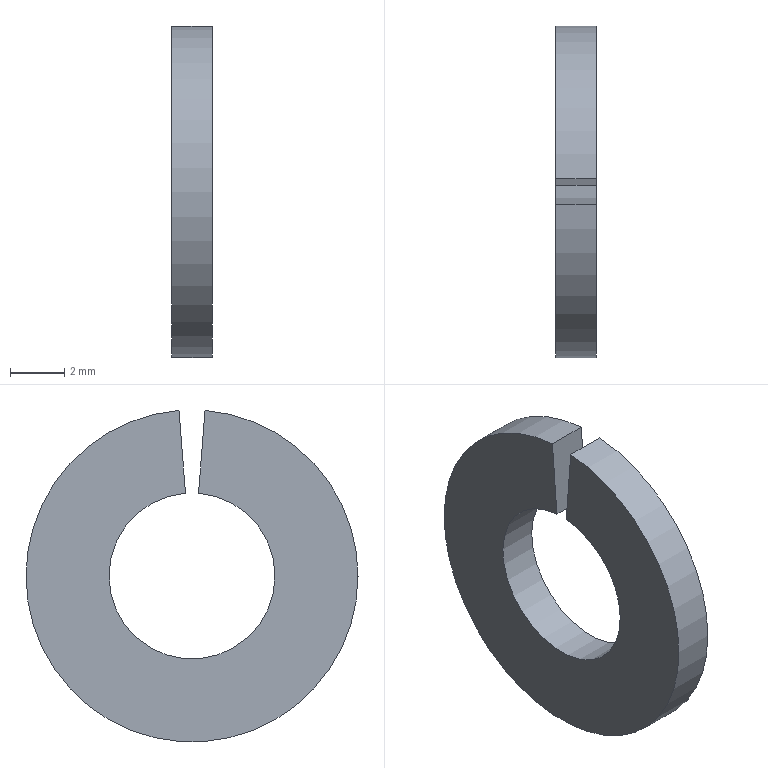Part | STEP file | PN_0038_default | 1 solid | 6 faces | box 1.5 x 12.2 x 12.181 mm | volume 128.223 mm3 | plane 4 | cylinder 2 | commonest cylinder face diameters 6.1 x1 12.2 x1
STEP:
#1=CARTESIAN_POINT('',(0.,0.,0.));
#2=DIRECTION('',(0.,0.,1.));
#3=DIRECTION('',(1.,0.,0.));
#4=AXIS2_PLACEMENT_3D('',#1,#2,#3);
#5=CARTESIAN_POINT('',(0.,0.2393,3.041));
#6=VERTEX_POINT('',#5);
#7=CARTESIAN_POINT('',(0.,0.4786,6.081));
#8=VERTEX_POINT('',#7);
#9=CARTESIAN_POINT('',(0.,0.2393,3.041));
#10=DIRECTION('',(0.,0.07846,0.9969));
#11=VECTOR('',#10,1.);
#12=LINE('',#9,#11);
#13=CARTESIAN_POINT('',(0.,3.05,0.));
#14=DIRECTION('',(-1.,0.,0.));
#15=DIRECTION('',(0.,0.,1.));
#16=AXIS2_PLACEMENT_3D('',#13,#14,#15);
#17=PLANE('',#16);
#18=CARTESIAN_POINT('',(3.041,-2.811));
#19=DIRECTION('',(0.9969,0.07846));
#20=VECTOR('',#19,1.);
#21=LINE('',#18,#20);
#22=(GEOMETRIC_REPRESENTATION_CONTEXT(2)PARAMETRIC_REPRESENTATION_CONTEXT()REPRESENTATION_CONTEXT('',''));
#23=DEFINITIONAL_REPRESENTATION('',(#21),#22);
#24=PCURVE('',#17,#23);
#25=CARTESIAN_POINT('',(-1.5,0.,0.));
#26=DIRECTION('',(0.,0.9969,-0.07846));
#27=DIRECTION('',(0.,0.07846,0.9969));
#28=AXIS2_PLACEMENT_3D('',#25,#26,#27);
#29=PLANE('',#28);
#30=CARTESIAN_POINT('',(3.05,1.5));
#31=DIRECTION('',(1.,0.));
#32=VECTOR('',#31,1.);
#33=LINE('',#30,#32);
#34=(GEOMETRIC_REPRESENTATION_CONTEXT(2)PARAMETRIC_REPRESENTATION_CONTEXT()REPRESENTATION_CONTEXT('',''));
#35=DEFINITIONAL_REPRESENTATION('',(#33),#34);
#36=PCURVE('',#29,#35);
#37=SURFACE_CURVE('',#12,(#24,#36),.PCURVE_S1.);
#38=EDGE_CURVE('',#6,#8,#37,.T.);
#39=ORIENTED_EDGE('',*,*,#38,.F.);
#40=CARTESIAN_POINT('',(0.,-0.2393,3.041));
#41=VERTEX_POINT('',#40);
#42=CARTESIAN_POINT('',(0.,0.,0.));
#43=DIRECTION('',(1.,0.,0.));
#44=DIRECTION('',(0.,0.,1.));
#45=AXIS2_PLACEMENT_3D('',#42,#43,#44);
#46=CIRCLE('',#45,3.05);
#47=CARTESIAN_POINT('',(3.05,-3.05));
#48=CARTESIAN_POINT('',(3.05,-8.333));
#49=CARTESIAN_POINT('',(-1.525,-5.691));
#50=CARTESIAN_POINT('',(-6.1,-3.05));
#51=CARTESIAN_POINT('',(-1.525,-0.4086));
#52=CARTESIAN_POINT('',(3.05,2.233));
#53=CARTESIAN_POINT('',(3.05,-3.05));
#54=(BOUNDED_CURVE()B_SPLINE_CURVE(2,(#47,#48,#49,#50,#51,#52,#53),.UNSPECIFIED.,.T.,.F.)B_SPLINE_CURVE_WITH_KNOTS((1,2,2,2,2,1),(-2.094,0.,2.094,4.189,6.283,8.378),.UNSPECIFIED.)CURVE()GEOMETRIC_REPRESENTATION_ITEM()RATIONAL_B_SPLINE_CURVE((1.,0.5,1.,0.5,1.,0.5,1.))REPRESENTATION_ITEM(''));
#55=(GEOMETRIC_REPRESENTATION_CONTEXT(2)PARAMETRIC_REPRESENTATION_CONTEXT()REPRESENTATION_CONTEXT('',''));
#56=DEFINITIONAL_REPRESENTATION('',(#54),#55);
#57=PCURVE('',#17,#56);
#58=CARTESIAN_POINT('',(-34.925,0.,0.));
#59=DIRECTION('',(-1.,0.,0.));
#60=DIRECTION('',(0.,0.,1.));
#61=AXIS2_PLACEMENT_3D('',#58,#59,#60);
#62=CYLINDRICAL_SURFACE('',#61,3.05);
#63=CARTESIAN_POINT('',(6.283,-34.925));
#64=DIRECTION('',(-1.,0.));
#65=VECTOR('',#64,1.);
#66=LINE('',#63,#65);
#67=(GEOMETRIC_REPRESENTATION_CONTEXT(2)PARAMETRIC_REPRESENTATION_CONTEXT()REPRESENTATION_CONTEXT('',''));
#68=DEFINITIONAL_REPRESENTATION('',(#66),#67);
#69=PCURVE('',#62,#68);
#70=SURFACE_CURVE('',#46,(#57,#69),.PCURVE_S1.);
#71=EDGE_CURVE('',#41,#6,#70,.T.);
#72=ORIENTED_EDGE('',*,*,#71,.F.);
#73=CARTESIAN_POINT('',(0.,-0.4786,6.081));
#74=VERTEX_POINT('',#73);
#75=CARTESIAN_POINT('',(0.,-0.4786,6.081));
#76=DIRECTION('',(0.,0.07846,-0.9969));
#77=VECTOR('',#76,1.);
#78=LINE('',#75,#77);
#79=CARTESIAN_POINT('',(6.081,-3.529));
#80=DIRECTION('',(-0.9969,0.07846));
#81=VECTOR('',#80,1.);
#82=LINE('',#79,#81);
#83=(GEOMETRIC_REPRESENTATION_CONTEXT(2)PARAMETRIC_REPRESENTATION_CONTEXT()REPRESENTATION_CONTEXT('',''));
#84=DEFINITIONAL_REPRESENTATION('',(#82),#83);
#85=PCURVE('',#17,#84);
#86=CARTESIAN_POINT('',(-1.5,0.,0.));
#87=DIRECTION('',(0.,0.9969,0.07846));
#88=DIRECTION('',(0.,-0.07846,0.9969));
#89=AXIS2_PLACEMENT_3D('',#86,#87,#88);
#90=PLANE('',#89);
#91=CARTESIAN_POINT('',(6.1,1.5));
#92=DIRECTION('',(-1.,0.));
#93=VECTOR('',#92,1.);
#94=LINE('',#91,#93);
#95=(GEOMETRIC_REPRESENTATION_CONTEXT(2)PARAMETRIC_REPRESENTATION_CONTEXT()REPRESENTATION_CONTEXT('',''));
#96=DEFINITIONAL_REPRESENTATION('',(#94),#95);
#97=PCURVE('',#90,#96);
#98=SURFACE_CURVE('',#78,(#85,#97),.PCURVE_S1.);
#99=EDGE_CURVE('',#74,#41,#98,.T.);
#100=ORIENTED_EDGE('',*,*,#99,.F.);
#101=CARTESIAN_POINT('',(0.,0.,0.));
#102=DIRECTION('',(-1.,0.,0.));
#103=DIRECTION('',(0.,0.,1.));
#104=AXIS2_PLACEMENT_3D('',#101,#102,#103);
#105=CIRCLE('',#104,6.1);
#106=CARTESIAN_POINT('',(0.,-3.05));
#107=DIRECTION('',(1.,0.));
#108=AXIS2_PLACEMENT_2D('',#106,#107);
#109=CIRCLE('',#108,6.1);
#110=(GEOMETRIC_REPRESENTATION_CONTEXT(2)PARAMETRIC_REPRESENTATION_CONTEXT()REPRESENTATION_CONTEXT('',''));
#111=DEFINITIONAL_REPRESENTATION('',(#109),#110);
#112=PCURVE('',#17,#111);
#113=CARTESIAN_POINT('',(-34.925,0.,0.));
#114=DIRECTION('',(-1.,0.,0.));
#115=DIRECTION('',(0.,0.,1.));
#116=AXIS2_PLACEMENT_3D('',#113,#114,#115);
#117=CYLINDRICAL_SURFACE('',#116,6.1);
#118=CARTESIAN_POINT('',(0.,-34.925));
#119=DIRECTION('',(1.,0.));
#120=VECTOR('',#119,1.);
#121=LINE('',#118,#120);
#122=(GEOMETRIC_REPRESENTATION_CONTEXT(2)PARAMETRIC_REPRESENTATION_CONTEXT()REPRESENTATION_CONTEXT('',''));
#123=DEFINITIONAL_REPRESENTATION('',(#121),#122);
#124=PCURVE('',#117,#123);
#125=SURFACE_CURVE('',#105,(#112,#124),.PCURVE_S1.);
#126=EDGE_CURVE('',#8,#74,#125,.T.);
#127=ORIENTED_EDGE('',*,*,#126,.F.);
#128=EDGE_LOOP('',(#39,#72,#100,#127));
#129=FACE_BOUND('',#128,.T.);
#130=ADVANCED_FACE('',(#129),#17,.F.);
#131=ORIENTED_EDGE('',*,*,#126,.T.);
#132=CARTESIAN_POINT('',(-1.5,-0.4786,6.081));
#133=VERTEX_POINT('',#132);
#134=CARTESIAN_POINT('',(-34.925,-0.4786,6.081));
#135=DIRECTION('',(-1.,0.,0.));
#136=VECTOR('',#135,1.);
#137=LINE('',#134,#136);
#138=CARTESIAN_POINT('',(6.205,0.));
#139=DIRECTION('',(0.,1.));
#140=VECTOR('',#139,1.);
#141=LINE('',#138,#140);
#142=(GEOMETRIC_REPRESENTATION_CONTEXT(2)PARAMETRIC_REPRESENTATION_CONTEXT()REPRESENTATION_CONTEXT('',''));
#143=DEFINITIONAL_REPRESENTATION('',(#141),#142);
#144=PCURVE('',#117,#143);
#145=CARTESIAN_POINT('',(6.1,-33.425));
#146=DIRECTION('',(0.,-1.));
#147=VECTOR('',#146,1.);
#148=LINE('',#145,#147);
#149=(GEOMETRIC_REPRESENTATION_CONTEXT(2)PARAMETRIC_REPRESENTATION_CONTEXT()REPRESENTATION_CONTEXT('',''));
#150=DEFINITIONAL_REPRESENTATION('',(#148),#149);
#151=PCURVE('',#90,#150);
#152=SURFACE_CURVE('',#137,(#144,#151),.PCURVE_S1.);
#153=EDGE_CURVE('',#74,#133,#152,.T.);
#154=ORIENTED_EDGE('',*,*,#153,.T.);
#155=CARTESIAN_POINT('',(-1.5,0.4786,6.081));
#156=VERTEX_POINT('',#155);
#157=CARTESIAN_POINT('',(-1.5,0.,0.));
#158=DIRECTION('',(1.,0.,0.));
#159=DIRECTION('',(0.,0.,1.));
#160=AXIS2_PLACEMENT_3D('',#157,#158,#159);
#161=CIRCLE('',#160,6.1);
#162=CARTESIAN_POINT('',(6.283,-33.425));
#163=DIRECTION('',(-1.,0.));
#164=VECTOR('',#163,1.);
#165=LINE('',#162,#164);
#166=(GEOMETRIC_REPRESENTATION_CONTEXT(2)PARAMETRIC_REPRESENTATION_CONTEXT()REPRESENTATION_CONTEXT('',''));
#167=DEFINITIONAL_REPRESENTATION('',(#165),#166);
#168=PCURVE('',#117,#167);
#169=CARTESIAN_POINT('',(-1.5,6.1,0.));
#170=DIRECTION('',(1.,0.,0.));
#171=DIRECTION('',(0.,0.,-1.));
#172=AXIS2_PLACEMENT_3D('',#169,#170,#171);
#173=PLANE('',#172);
#174=CARTESIAN_POINT('',(0.,-6.1));
#175=DIRECTION('',(-1.,0.));
#176=AXIS2_PLACEMENT_2D('',#174,#175);
#177=CIRCLE('',#176,6.1);
#178=(GEOMETRIC_REPRESENTATION_CONTEXT(2)PARAMETRIC_REPRESENTATION_CONTEXT()REPRESENTATION_CONTEXT('',''));
#179=DEFINITIONAL_REPRESENTATION('',(#177),#178);
#180=PCURVE('',#173,#179);
#181=SURFACE_CURVE('',#161,(#168,#180),.PCURVE_S1.);
#182=EDGE_CURVE('',#133,#156,#181,.T.);
#183=ORIENTED_EDGE('',*,*,#182,.T.);
#184=CARTESIAN_POINT('',(-34.925,0.4786,6.081));
#185=DIRECTION('',(1.,0.,0.));
#186=VECTOR('',#185,1.);
#187=LINE('',#184,#186);
#188=CARTESIAN_POINT('',(0.07854,0.));
#189=DIRECTION('',(0.,-1.));
#190=VECTOR('',#189,1.);
#191=LINE('',#188,#190);
#192=(GEOMETRIC_REPRESENTATION_CONTEXT(2)PARAMETRIC_REPRESENTATION_CONTEXT()REPRESENTATION_CONTEXT('',''));
#193=DEFINITIONAL_REPRESENTATION('',(#191),#192);
#194=PCURVE('',#117,#193);
#195=CARTESIAN_POINT('',(6.1,-33.425));
#196=DIRECTION('',(0.,1.));
#197=VECTOR('',#196,1.);
#198=LINE('',#195,#197);
#199=(GEOMETRIC_REPRESENTATION_CONTEXT(2)PARAMETRIC_REPRESENTATION_CONTEXT()REPRESENTATION_CONTEXT('',''));
#200=DEFINITIONAL_REPRESENTATION('',(#198),#199);
#201=PCURVE('',#29,#200);
#202=SURFACE_CURVE('',#187,(#194,#201),.PCURVE_S1.);
#203=EDGE_CURVE('',#156,#8,#202,.T.);
#204=ORIENTED_EDGE('',*,*,#203,.T.);
#205=EDGE_LOOP('',(#131,#154,#183,#204));
#206=FACE_BOUND('',#205,.T.);
#207=ADVANCED_FACE('',(#206),#117,.T.);
#208=ORIENTED_EDGE('',*,*,#203,.F.);
#209=CARTESIAN_POINT('',(-1.5,0.2393,3.041));
#210=VERTEX_POINT('',#209);
#211=CARTESIAN_POINT('',(-1.5,0.,0.));
#212=DIRECTION('',(0.,0.07846,0.9969));
#213=VECTOR('',#212,1.);
#214=LINE('',#211,#213);
#215=CARTESIAN_POINT('',(0.,0.));
#216=DIRECTION('',(1.,0.));
#217=VECTOR('',#216,1.);
#218=LINE('',#215,#217);
#219=(GEOMETRIC_REPRESENTATION_CONTEXT(2)PARAMETRIC_REPRESENTATION_CONTEXT()REPRESENTATION_CONTEXT('',''));
#220=DEFINITIONAL_REPRESENTATION('',(#218),#219);
#221=PCURVE('',#29,#220);
#222=CARTESIAN_POINT('',(0.,-6.1));
#223=DIRECTION('',(-0.9969,0.07846));
#224=VECTOR('',#223,1.);
#225=LINE('',#222,#224);
#226=(GEOMETRIC_REPRESENTATION_CONTEXT(2)PARAMETRIC_REPRESENTATION_CONTEXT()REPRESENTATION_CONTEXT('',''));
#227=DEFINITIONAL_REPRESENTATION('',(#225),#226);
#228=PCURVE('',#173,#227);
#229=SURFACE_CURVE('',#214,(#221,#228),.PCURVE_S1.);
#230=EDGE_CURVE('',#210,#156,#229,.T.);
#231=ORIENTED_EDGE('',*,*,#230,.F.);
#232=CARTESIAN_POINT('',(-1.5,0.2393,3.041));
#233=DIRECTION('',(-1.,0.,0.));
#234=VECTOR('',#233,1.);
#235=LINE('',#232,#234);
#236=CARTESIAN_POINT('',(3.05,0.));
#237=DIRECTION('',(0.,-1.));
#238=VECTOR('',#237,1.);
#239=LINE('',#236,#238);
#240=(GEOMETRIC_REPRESENTATION_CONTEXT(2)PARAMETRIC_REPRESENTATION_CONTEXT()REPRESENTATION_CONTEXT('',''));
#241=DEFINITIONAL_REPRESENTATION('',(#239),#240);
#242=PCURVE('',#29,#241);
#243=CARTESIAN_POINT('',(0.07854,-33.425));
#244=DIRECTION('',(0.,1.));
#245=VECTOR('',#244,1.);
#246=LINE('',#243,#245);
#247=(GEOMETRIC_REPRESENTATION_CONTEXT(2)PARAMETRIC_REPRESENTATION_CONTEXT()REPRESENTATION_CONTEXT('',''));
#248=DEFINITIONAL_REPRESENTATION('',(#246),#247);
#249=PCURVE('',#62,#248);
#250=SURFACE_CURVE('',#235,(#242,#249),.PCURVE_S1.);
#251=EDGE_CURVE('',#6,#210,#250,.T.);
#252=ORIENTED_EDGE('',*,*,#251,.F.);
#253=ORIENTED_EDGE('',*,*,#38,.T.);
#254=EDGE_LOOP('',(#208,#231,#252,#253));
#255=FACE_BOUND('',#254,.T.);
#256=ADVANCED_FACE('',(#255),#29,.F.);
#257=ORIENTED_EDGE('',*,*,#71,.F.);
#258=CARTESIAN_POINT('',(-1.5,-0.2393,3.041));
#259=VERTEX_POINT('',#258);
#260=CARTESIAN_POINT('',(-34.925,-0.2393,3.041));
#261=DIRECTION('',(-1.,0.,0.));
#262=VECTOR('',#261,1.);
#263=LINE('',#260,#262);
#264=CARTESIAN_POINT('',(6.205,0.));
#265=DIRECTION('',(0.,1.));
#266=VECTOR('',#265,1.);
#267=LINE('',#264,#266);
#268=(GEOMETRIC_REPRESENTATION_CONTEXT(2)PARAMETRIC_REPRESENTATION_CONTEXT()REPRESENTATION_CONTEXT('',''));
#269=DEFINITIONAL_REPRESENTATION('',(#267),#268);
#270=PCURVE('',#62,#269);
#271=CARTESIAN_POINT('',(3.05,-33.425));
#272=DIRECTION('',(0.,-1.));
#273=VECTOR('',#272,1.);
#274=LINE('',#271,#273);
#275=(GEOMETRIC_REPRESENTATION_CONTEXT(2)PARAMETRIC_REPRESENTATION_CONTEXT()REPRESENTATION_CONTEXT('',''));
#276=DEFINITIONAL_REPRESENTATION('',(#274),#275);
#277=PCURVE('',#90,#276);
#278=SURFACE_CURVE('',#263,(#270,#277),.PCURVE_S1.);
#279=EDGE_CURVE('',#41,#259,#278,.T.);
#280=ORIENTED_EDGE('',*,*,#279,.T.);
#281=CARTESIAN_POINT('',(-1.5,0.,0.));
#282=DIRECTION('',(1.,0.,0.));
#283=DIRECTION('',(0.,0.,1.));
#284=AXIS2_PLACEMENT_3D('',#281,#282,#283);
#285=CIRCLE('',#284,3.05);
#286=CARTESIAN_POINT('',(6.283,-33.425));
#287=DIRECTION('',(-1.,0.));
#288=VECTOR('',#287,1.);
#289=LINE('',#286,#288);
#290=(GEOMETRIC_REPRESENTATION_CONTEXT(2)PARAMETRIC_REPRESENTATION_CONTEXT()REPRESENTATION_CONTEXT('',''));
#291=DEFINITIONAL_REPRESENTATION('',(#289),#290);
#292=PCURVE('',#62,#291);
#293=CARTESIAN_POINT('',(0.,-6.1));
#294=DIRECTION('',(-1.,0.));
#295=AXIS2_PLACEMENT_2D('',#293,#294);
#296=CIRCLE('',#295,3.05);
#297=(GEOMETRIC_REPRESENTATION_CONTEXT(2)PARAMETRIC_REPRESENTATION_CONTEXT()REPRESENTATION_CONTEXT('',''));
#298=DEFINITIONAL_REPRESENTATION('',(#296),#297);
#299=PCURVE('',#173,#298);
#300=SURFACE_CURVE('',#285,(#292,#299),.PCURVE_S1.);
#301=EDGE_CURVE('',#259,#210,#300,.T.);
#302=ORIENTED_EDGE('',*,*,#301,.T.);
#303=ORIENTED_EDGE('',*,*,#251,.F.);
#304=EDGE_LOOP('',(#257,#280,#302,#303));
#305=FACE_BOUND('',#304,.F.);
#306=ADVANCED_FACE('',(#305),#62,.F.);
#307=ORIENTED_EDGE('',*,*,#153,.F.);
#308=ORIENTED_EDGE('',*,*,#99,.T.);
#309=ORIENTED_EDGE('',*,*,#279,.T.);
#310=CARTESIAN_POINT('',(-1.5,0.,0.));
#311=DIRECTION('',(0.,-0.07846,0.9969));
#312=VECTOR('',#311,1.);
#313=LINE('',#310,#312);
#314=CARTESIAN_POINT('',(0.,0.));
#315=DIRECTION('',(1.,0.));
#316=VECTOR('',#315,1.);
#317=LINE('',#314,#316);
#318=(GEOMETRIC_REPRESENTATION_CONTEXT(2)PARAMETRIC_REPRESENTATION_CONTEXT()REPRESENTATION_CONTEXT('',''));
#319=DEFINITIONAL_REPRESENTATION('',(#317),#318);
#320=PCURVE('',#90,#319);
#321=CARTESIAN_POINT('',(0.,-6.1));
#322=DIRECTION('',(-0.9969,-0.07846));
#323=VECTOR('',#322,1.);
#324=LINE('',#321,#323);
#325=(GEOMETRIC_REPRESENTATION_CONTEXT(2)PARAMETRIC_REPRESENTATION_CONTEXT()REPRESENTATION_CONTEXT('',''));
#326=DEFINITIONAL_REPRESENTATION('',(#324),#325);
#327=PCURVE('',#173,#326);
#328=SURFACE_CURVE('',#313,(#320,#327),.PCURVE_S1.);
#329=EDGE_CURVE('',#259,#133,#328,.T.);
#330=ORIENTED_EDGE('',*,*,#329,.T.);
#331=EDGE_LOOP('',(#307,#308,#309,#330));
#332=FACE_BOUND('',#331,.T.);
#333=ADVANCED_FACE('',(#332),#90,.T.);
#334=ORIENTED_EDGE('',*,*,#230,.T.);
#335=ORIENTED_EDGE('',*,*,#182,.F.);
#336=ORIENTED_EDGE('',*,*,#329,.F.);
#337=ORIENTED_EDGE('',*,*,#301,.T.);
#338=EDGE_LOOP('',(#334,#335,#336,#337));
#339=FACE_BOUND('',#338,.T.);
#340=ADVANCED_FACE('',(#339),#173,.F.);
#341=CLOSED_SHELL('',(#130,#207,#256,#306,#333,#340));
#342=MANIFOLD_SOLID_BREP('',#341);
#343=(LENGTH_UNIT()NAMED_UNIT(*)SI_UNIT(.MILLI.,.METRE.));
#344=UNCERTAINTY_MEASURE_WITH_UNIT(LENGTH_MEASURE(0.0000001),#343,'','');
#345=(NAMED_UNIT(*)PLANE_ANGLE_UNIT()SI_UNIT($,.RADIAN.));
#346=(NAMED_UNIT(*)SI_UNIT($,.STERADIAN.)SOLID_ANGLE_UNIT());
#347=(GEOMETRIC_REPRESENTATION_CONTEXT(3)GLOBAL_UNCERTAINTY_ASSIGNED_CONTEXT((#344))GLOBAL_UNIT_ASSIGNED_CONTEXT((#343,#345,#346))REPRESENTATION_CONTEXT('',''));
#348=ADVANCED_BREP_SHAPE_REPRESENTATION('',(#4,#342),#347);